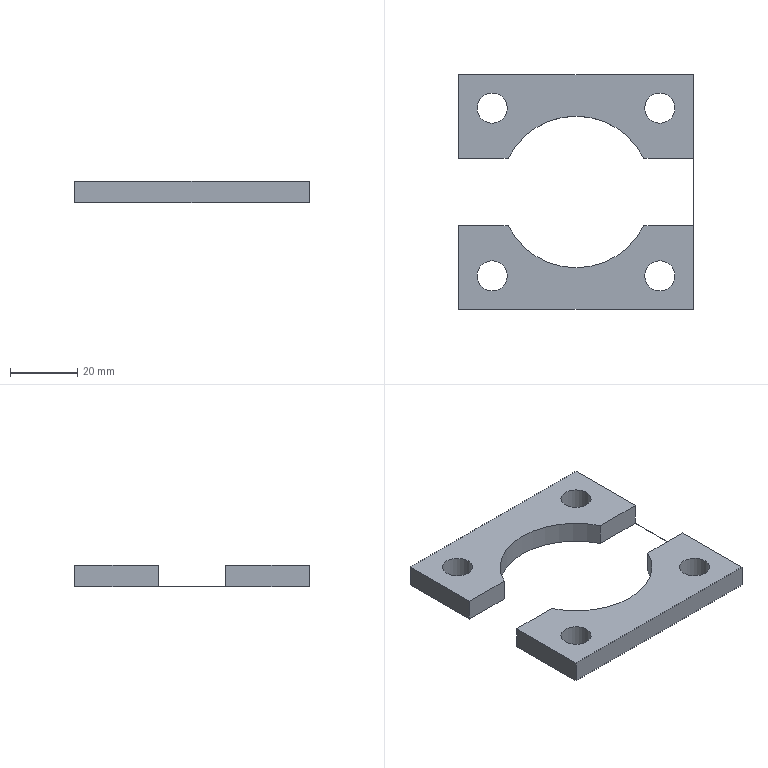Part | NX | features solid 2 | 1 solid | 20 faces | box 70 x 70 x 6.5 mm | volume 16344 mm3 | plane 14 | cylinder 6 | commonest cylinder face diameters 9 x4 45.2 x2
STEP:
#1=CARTESIAN_POINT('',(-460.,-390.,-210.));
#2=VERTEX_POINT('',#1);
#3=CARTESIAN_POINT('',(-390.,-390.,-210.));
#4=VERTEX_POINT('',#3);
#5=CARTESIAN_POINT('',(-460.,-390.,-210.));
#6=DIRECTION('',(1.,0.,0.));
#7=VECTOR('',#6,1000.);
#8=LINE('',#5,#7);
#9=EDGE_CURVE('',#2,#4,#8,.T.);
#10=ORIENTED_EDGE('',*,*,#9,.T.);
#11=CARTESIAN_POINT('',(-390.,-390.,-203.5));
#12=VERTEX_POINT('',#11);
#13=CARTESIAN_POINT('',(-390.,-390.,-203.5));
#14=DIRECTION('',(0.,0.,-1.));
#15=VECTOR('',#14,1000.);
#16=LINE('',#13,#15);
#17=EDGE_CURVE('',#12,#4,#16,.T.);
#18=ORIENTED_EDGE('',*,*,#17,.F.);
#19=CARTESIAN_POINT('',(-460.,-390.,-203.5));
#20=VERTEX_POINT('',#19);
#21=CARTESIAN_POINT('',(-460.,-390.,-203.5));
#22=DIRECTION('',(1.,0.,0.));
#23=VECTOR('',#22,1000.);
#24=LINE('',#21,#23);
#25=EDGE_CURVE('',#20,#12,#24,.T.);
#26=ORIENTED_EDGE('',*,*,#25,.F.);
#27=CARTESIAN_POINT('',(-460.,-390.,-203.5));
#28=DIRECTION('',(0.,0.,-1.));
#29=VECTOR('',#28,1000.);
#30=LINE('',#27,#29);
#31=EDGE_CURVE('',#20,#2,#30,.T.);
#32=ORIENTED_EDGE('',*,*,#31,.T.);
#33=EDGE_LOOP('',(#10,#18,#26,#32));
#34=FACE_BOUND('',#33,.T.);
#35=CARTESIAN_POINT('',(-460.,-390.,-203.5));
#36=DIRECTION('',(0.,1.,0.));
#37=DIRECTION('',(0.,0.,1.));
#38=AXIS2_PLACEMENT_3D('',#35,#36,#37);
#39=PLANE('',#38);
#40=ADVANCED_FACE('',(#34),#39,.F.);
#41=CARTESIAN_POINT('',(-390.,-320.,-210.));
#42=VERTEX_POINT('',#41);
#43=CARTESIAN_POINT('',(-390.,-390.,-210.));
#44=DIRECTION('',(0.,1.,0.));
#45=VECTOR('',#44,1000.);
#46=LINE('',#43,#45);
#47=EDGE_CURVE('',#4,#42,#46,.T.);
#48=ORIENTED_EDGE('',*,*,#47,.T.);
#49=CARTESIAN_POINT('',(-390.,-320.,-203.5));
#50=VERTEX_POINT('',#49);
#51=CARTESIAN_POINT('',(-390.,-320.,-210.));
#52=DIRECTION('',(0.,0.,-1.));
#53=VECTOR('',#52,1000.);
#54=LINE('',#51,#53);
#55=EDGE_CURVE('',#50,#42,#54,.T.);
#56=ORIENTED_EDGE('',*,*,#55,.F.);
#57=CARTESIAN_POINT('',(-390.,-345.,-203.5));
#58=VERTEX_POINT('',#57);
#59=CARTESIAN_POINT('',(-390.,-345.,-203.5));
#60=DIRECTION('',(0.,1.,0.));
#61=VECTOR('',#60,1000.);
#62=LINE('',#59,#61);
#63=EDGE_CURVE('',#58,#50,#62,.T.);
#64=ORIENTED_EDGE('',*,*,#63,.F.);
#65=CARTESIAN_POINT('',(-390.,-345.,-209.99));
#66=VERTEX_POINT('',#65);
#67=CARTESIAN_POINT('',(-390.,-345.,-203.5));
#68=DIRECTION('',(0.,0.,-1.));
#69=VECTOR('',#68,1000.);
#70=LINE('',#67,#69);
#71=EDGE_CURVE('',#58,#66,#70,.T.);
#72=ORIENTED_EDGE('',*,*,#71,.T.);
#73=CARTESIAN_POINT('',(-390.,-365.,-209.99));
#74=VERTEX_POINT('',#73);
#75=CARTESIAN_POINT('',(-390.,-390.,-209.99));
#76=DIRECTION('',(0.,-1.,0.));
#77=VECTOR('',#76,1000.);
#78=LINE('',#75,#77);
#79=EDGE_CURVE('',#74,#66,#78,.F.);
#80=ORIENTED_EDGE('',*,*,#79,.F.);
#81=CARTESIAN_POINT('',(-390.,-365.,-203.5));
#82=VERTEX_POINT('',#81);
#83=CARTESIAN_POINT('',(-390.,-365.,-203.5));
#84=DIRECTION('',(0.,0.,-1.));
#85=VECTOR('',#84,1000.);
#86=LINE('',#83,#85);
#87=EDGE_CURVE('',#82,#74,#86,.T.);
#88=ORIENTED_EDGE('',*,*,#87,.F.);
#89=CARTESIAN_POINT('',(-390.,-390.,-203.5));
#90=DIRECTION('',(0.,1.,0.));
#91=VECTOR('',#90,1000.);
#92=LINE('',#89,#91);
#93=EDGE_CURVE('',#12,#82,#92,.T.);
#94=ORIENTED_EDGE('',*,*,#93,.F.);
#95=ORIENTED_EDGE('',*,*,#17,.T.);
#96=EDGE_LOOP('',(#48,#56,#64,#72,#80,#88,#94,#95));
#97=FACE_BOUND('',#96,.T.);
#98=CARTESIAN_POINT('',(-390.,-390.,-203.5));
#99=DIRECTION('',(-1.,0.,0.));
#100=DIRECTION('',(0.,0.,-1.));
#101=AXIS2_PLACEMENT_3D('',#98,#99,#100);
#102=PLANE('',#101);
#103=ADVANCED_FACE('',(#97),#102,.F.);
#104=CARTESIAN_POINT('',(-390.01,-365.,-209.99));
#105=VERTEX_POINT('',#104);
#106=CARTESIAN_POINT('',(-390.,-365.,-209.99));
#107=DIRECTION('',(-1.,0.,0.));
#108=VECTOR('',#107,1000.);
#109=LINE('',#106,#108);
#110=EDGE_CURVE('',#74,#105,#109,.T.);
#111=ORIENTED_EDGE('',*,*,#110,.T.);
#112=CARTESIAN_POINT('',(-390.01,-365.,-210.));
#113=VERTEX_POINT('',#112);
#114=CARTESIAN_POINT('',(-390.01,-365.,-203.5));
#115=DIRECTION('',(0.,0.,1.));
#116=VECTOR('',#115,1000.);
#117=LINE('',#114,#116);
#118=EDGE_CURVE('',#105,#113,#117,.F.);
#119=ORIENTED_EDGE('',*,*,#118,.T.);
#120=CARTESIAN_POINT('',(-404.733,-365.,-210.));
#121=VERTEX_POINT('',#120);
#122=CARTESIAN_POINT('',(-390.,-365.,-210.));
#123=DIRECTION('',(-1.,0.,0.));
#124=VECTOR('',#123,1000.);
#125=LINE('',#122,#124);
#126=EDGE_CURVE('',#113,#121,#125,.T.);
#127=ORIENTED_EDGE('',*,*,#126,.T.);
#128=CARTESIAN_POINT('',(-404.733,-365.,-203.5));
#129=VERTEX_POINT('',#128);
#130=CARTESIAN_POINT('',(-404.733,-365.,-203.5));
#131=DIRECTION('',(0.,0.,-1.));
#132=VECTOR('',#131,1000.);
#133=LINE('',#130,#132);
#134=EDGE_CURVE('',#129,#121,#133,.T.);
#135=ORIENTED_EDGE('',*,*,#134,.F.);
#136=CARTESIAN_POINT('',(-390.,-365.,-203.5));
#137=DIRECTION('',(-1.,0.,0.));
#138=VECTOR('',#137,1000.);
#139=LINE('',#136,#138);
#140=EDGE_CURVE('',#82,#129,#139,.T.);
#141=ORIENTED_EDGE('',*,*,#140,.F.);
#142=ORIENTED_EDGE('',*,*,#87,.T.);
#143=EDGE_LOOP('',(#111,#119,#127,#135,#141,#142));
#144=FACE_BOUND('',#143,.T.);
#145=CARTESIAN_POINT('',(-390.,-365.,-203.5));
#146=DIRECTION('',(0.,-1.,0.));
#147=DIRECTION('',(1.,0.,0.));
#148=AXIS2_PLACEMENT_3D('',#145,#146,#147);
#149=PLANE('',#148);
#150=ADVANCED_FACE('',(#144),#149,.F.);
#151=CARTESIAN_POINT('',(-445.267,-365.,-210.));
#152=VERTEX_POINT('',#151);
#153=CARTESIAN_POINT('',(-425.,-355.,-210.));
#154=DIRECTION('',(0.,0.,1.));
#155=DIRECTION('',(0.,-1.,0.));
#156=AXIS2_PLACEMENT_3D('',#153,#154,#155);
#157=CIRCLE('',#156,22.6);
#158=EDGE_CURVE('',#152,#121,#157,.T.);
#159=ORIENTED_EDGE('',*,*,#158,.F.);
#160=CARTESIAN_POINT('',(-445.267,-365.,-203.5));
#161=VERTEX_POINT('',#160);
#162=CARTESIAN_POINT('',(-445.267,-365.,-203.5));
#163=DIRECTION('',(0.,0.,-1.));
#164=VECTOR('',#163,1000.);
#165=LINE('',#162,#164);
#166=EDGE_CURVE('',#161,#152,#165,.T.);
#167=ORIENTED_EDGE('',*,*,#166,.F.);
#168=CARTESIAN_POINT('',(-425.,-355.,-203.5));
#169=DIRECTION('',(0.,0.,1.));
#170=DIRECTION('',(0.,-1.,0.));
#171=AXIS2_PLACEMENT_3D('',#168,#169,#170);
#172=CIRCLE('',#171,22.6);
#173=EDGE_CURVE('',#161,#129,#172,.T.);
#174=ORIENTED_EDGE('',*,*,#173,.T.);
#175=ORIENTED_EDGE('',*,*,#134,.T.);
#176=EDGE_LOOP('',(#159,#167,#174,#175));
#177=FACE_BOUND('',#176,.T.);
#178=CARTESIAN_POINT('',(-425.,-355.,-203.5));
#179=DIRECTION('',(0.,0.,-1.));
#180=DIRECTION('',(0.,1.,0.));
#181=AXIS2_PLACEMENT_3D('',#178,#179,#180);
#182=CYLINDRICAL_SURFACE('',#181,22.6);
#183=ADVANCED_FACE('',(#177),#182,.F.);
#184=CARTESIAN_POINT('',(-460.,-365.,-210.));
#185=VERTEX_POINT('',#184);
#186=CARTESIAN_POINT('',(-445.267,-365.,-210.));
#187=DIRECTION('',(-1.,0.,0.));
#188=VECTOR('',#187,1000.);
#189=LINE('',#186,#188);
#190=EDGE_CURVE('',#152,#185,#189,.T.);
#191=ORIENTED_EDGE('',*,*,#190,.T.);
#192=CARTESIAN_POINT('',(-460.,-365.,-203.5));
#193=VERTEX_POINT('',#192);
#194=CARTESIAN_POINT('',(-460.,-365.,-203.5));
#195=DIRECTION('',(0.,0.,-1.));
#196=VECTOR('',#195,1000.);
#197=LINE('',#194,#196);
#198=EDGE_CURVE('',#193,#185,#197,.T.);
#199=ORIENTED_EDGE('',*,*,#198,.F.);
#200=CARTESIAN_POINT('',(-445.267,-365.,-203.5));
#201=DIRECTION('',(-1.,0.,0.));
#202=VECTOR('',#201,1000.);
#203=LINE('',#200,#202);
#204=EDGE_CURVE('',#161,#193,#203,.T.);
#205=ORIENTED_EDGE('',*,*,#204,.F.);
#206=ORIENTED_EDGE('',*,*,#166,.T.);
#207=EDGE_LOOP('',(#191,#199,#205,#206));
#208=FACE_BOUND('',#207,.T.);
#209=CARTESIAN_POINT('',(-445.267,-365.,-203.5));
#210=DIRECTION('',(0.,-1.,0.));
#211=DIRECTION('',(1.,0.,0.));
#212=AXIS2_PLACEMENT_3D('',#209,#210,#211);
#213=PLANE('',#212);
#214=ADVANCED_FACE('',(#208),#213,.F.);
#215=CARTESIAN_POINT('',(-450.,-384.5,-203.5));
#216=VERTEX_POINT('',#215);
#217=CARTESIAN_POINT('',(-450.,-380.,-203.5));
#218=DIRECTION('',(0.,0.,1.));
#219=DIRECTION('',(0.,-1.,0.));
#220=AXIS2_PLACEMENT_3D('',#217,#218,#219);
#221=CIRCLE('',#220,4.5);
#222=EDGE_CURVE('',#216,#216,#221,.T.);
#223=ORIENTED_EDGE('',*,*,#222,.T.);
#224=EDGE_LOOP('',(#223));
#225=FACE_BOUND('',#224,.T.);
#226=CARTESIAN_POINT('',(-450.,-384.5,-210.));
#227=VERTEX_POINT('',#226);
#228=CARTESIAN_POINT('',(-450.,-380.,-210.));
#229=DIRECTION('',(0.,0.,1.));
#230=DIRECTION('',(0.,-1.,0.));
#231=AXIS2_PLACEMENT_3D('',#228,#229,#230);
#232=CIRCLE('',#231,4.5);
#233=EDGE_CURVE('',#227,#227,#232,.T.);
#234=ORIENTED_EDGE('',*,*,#233,.F.);
#235=EDGE_LOOP('',(#234));
#236=FACE_BOUND('',#235,.T.);
#237=CARTESIAN_POINT('',(-450.,-380.,-203.5));
#238=DIRECTION('',(0.,0.,-1.));
#239=DIRECTION('',(0.,1.,0.));
#240=AXIS2_PLACEMENT_3D('',#237,#238,#239);
#241=CYLINDRICAL_SURFACE('',#240,4.5);
#242=ADVANCED_FACE('',(#225,#236),#241,.F.);
#243=CARTESIAN_POINT('',(-400.,-384.5,-203.5));
#244=VERTEX_POINT('',#243);
#245=CARTESIAN_POINT('',(-400.,-380.,-203.5));
#246=DIRECTION('',(0.,0.,1.));
#247=DIRECTION('',(0.,-1.,0.));
#248=AXIS2_PLACEMENT_3D('',#245,#246,#247);
#249=CIRCLE('',#248,4.5);
#250=EDGE_CURVE('',#244,#244,#249,.T.);
#251=ORIENTED_EDGE('',*,*,#250,.T.);
#252=EDGE_LOOP('',(#251));
#253=FACE_BOUND('',#252,.T.);
#254=CARTESIAN_POINT('',(-400.,-384.5,-210.));
#255=VERTEX_POINT('',#254);
#256=CARTESIAN_POINT('',(-400.,-380.,-210.));
#257=DIRECTION('',(0.,0.,1.));
#258=DIRECTION('',(0.,-1.,0.));
#259=AXIS2_PLACEMENT_3D('',#256,#257,#258);
#260=CIRCLE('',#259,4.5);
#261=EDGE_CURVE('',#255,#255,#260,.T.);
#262=ORIENTED_EDGE('',*,*,#261,.F.);
#263=EDGE_LOOP('',(#262));
#264=FACE_BOUND('',#263,.T.);
#265=CARTESIAN_POINT('',(-400.,-380.,-203.5));
#266=DIRECTION('',(0.,0.,-1.));
#267=DIRECTION('',(0.,1.,0.));
#268=AXIS2_PLACEMENT_3D('',#265,#266,#267);
#269=CYLINDRICAL_SURFACE('',#268,4.5);
#270=ADVANCED_FACE('',(#253,#264),#269,.F.);
#271=CARTESIAN_POINT('',(-460.,-365.,-210.));
#272=DIRECTION('',(0.,-1.,0.));
#273=VECTOR('',#272,1000.);
#274=LINE('',#271,#273);
#275=EDGE_CURVE('',#185,#2,#274,.T.);
#276=ORIENTED_EDGE('',*,*,#275,.T.);
#277=ORIENTED_EDGE('',*,*,#31,.F.);
#278=CARTESIAN_POINT('',(-460.,-365.,-203.5));
#279=DIRECTION('',(0.,-1.,0.));
#280=VECTOR('',#279,1000.);
#281=LINE('',#278,#280);
#282=EDGE_CURVE('',#193,#20,#281,.T.);
#283=ORIENTED_EDGE('',*,*,#282,.F.);
#284=ORIENTED_EDGE('',*,*,#198,.T.);
#285=EDGE_LOOP('',(#276,#277,#283,#284));
#286=FACE_BOUND('',#285,.T.);
#287=CARTESIAN_POINT('',(-460.,-365.,-203.5));
#288=DIRECTION('',(1.,0.,0.));
#289=DIRECTION('',(0.,0.,1.));
#290=AXIS2_PLACEMENT_3D('',#287,#288,#289);
#291=PLANE('',#290);
#292=ADVANCED_FACE('',(#286),#291,.F.);
#293=ORIENTED_EDGE('',*,*,#250,.F.);
#294=EDGE_LOOP('',(#293));
#295=FACE_BOUND('',#294,.T.);
#296=ORIENTED_EDGE('',*,*,#222,.F.);
#297=EDGE_LOOP('',(#296));
#298=FACE_BOUND('',#297,.T.);
#299=ORIENTED_EDGE('',*,*,#25,.T.);
#300=ORIENTED_EDGE('',*,*,#93,.T.);
#301=ORIENTED_EDGE('',*,*,#140,.T.);
#302=ORIENTED_EDGE('',*,*,#173,.F.);
#303=ORIENTED_EDGE('',*,*,#204,.T.);
#304=ORIENTED_EDGE('',*,*,#282,.T.);
#305=EDGE_LOOP('',(#299,#300,#301,#302,#303,#304));
#306=FACE_BOUND('',#305,.T.);
#307=CARTESIAN_POINT('',(-425.,-355.,-203.5));
#308=DIRECTION('',(0.,0.,1.));
#309=DIRECTION('',(0.,-1.,0.));
#310=AXIS2_PLACEMENT_3D('',#307,#308,#309);
#311=PLANE('',#310);
#312=ADVANCED_FACE('',(#295,#298,#306),#311,.T.);
#313=ORIENTED_EDGE('',*,*,#261,.T.);
#314=EDGE_LOOP('',(#313));
#315=FACE_BOUND('',#314,.T.);
#316=ORIENTED_EDGE('',*,*,#233,.T.);
#317=EDGE_LOOP('',(#316));
#318=FACE_BOUND('',#317,.T.);
#319=CARTESIAN_POINT('',(-390.01,-345.,-210.));
#320=VERTEX_POINT('',#319);
#321=CARTESIAN_POINT('',(-390.01,-390.,-210.));
#322=DIRECTION('',(0.,1.,0.));
#323=VECTOR('',#322,1000.);
#324=LINE('',#321,#323);
#325=EDGE_CURVE('',#113,#320,#324,.T.);
#326=ORIENTED_EDGE('',*,*,#325,.T.);
#327=CARTESIAN_POINT('',(-404.733,-345.,-210.));
#328=VERTEX_POINT('',#327);
#329=CARTESIAN_POINT('',(-390.,-345.,-210.));
#330=DIRECTION('',(-1.,0.,0.));
#331=VECTOR('',#330,1000.);
#332=LINE('',#329,#331);
#333=EDGE_CURVE('',#320,#328,#332,.T.);
#334=ORIENTED_EDGE('',*,*,#333,.T.);
#335=CARTESIAN_POINT('',(-445.267,-345.,-210.));
#336=VERTEX_POINT('',#335);
#337=CARTESIAN_POINT('',(-425.,-355.,-210.));
#338=DIRECTION('',(0.,0.,1.));
#339=DIRECTION('',(0.,-1.,0.));
#340=AXIS2_PLACEMENT_3D('',#337,#338,#339);
#341=CIRCLE('',#340,22.6);
#342=EDGE_CURVE('',#328,#336,#341,.T.);
#343=ORIENTED_EDGE('',*,*,#342,.T.);
#344=CARTESIAN_POINT('',(-460.,-345.,-210.));
#345=VERTEX_POINT('',#344);
#346=CARTESIAN_POINT('',(-445.267,-345.,-210.));
#347=DIRECTION('',(-1.,0.,0.));
#348=VECTOR('',#347,1000.);
#349=LINE('',#346,#348);
#350=EDGE_CURVE('',#336,#345,#349,.T.);
#351=ORIENTED_EDGE('',*,*,#350,.T.);
#352=CARTESIAN_POINT('',(-460.,-320.,-210.));
#353=VERTEX_POINT('',#352);
#354=CARTESIAN_POINT('',(-460.,-320.,-210.));
#355=DIRECTION('',(0.,-1.,0.));
#356=VECTOR('',#355,1000.);
#357=LINE('',#354,#356);
#358=EDGE_CURVE('',#353,#345,#357,.T.);
#359=ORIENTED_EDGE('',*,*,#358,.F.);
#360=CARTESIAN_POINT('',(-390.,-320.,-210.));
#361=DIRECTION('',(-1.,0.,0.));
#362=VECTOR('',#361,1000.);
#363=LINE('',#360,#362);
#364=EDGE_CURVE('',#42,#353,#363,.T.);
#365=ORIENTED_EDGE('',*,*,#364,.F.);
#366=ORIENTED_EDGE('',*,*,#47,.F.);
#367=ORIENTED_EDGE('',*,*,#9,.F.);
#368=ORIENTED_EDGE('',*,*,#275,.F.);
#369=ORIENTED_EDGE('',*,*,#190,.F.);
#370=ORIENTED_EDGE('',*,*,#158,.T.);
#371=ORIENTED_EDGE('',*,*,#126,.F.);
#372=EDGE_LOOP('',(#326,#334,#343,#351,#359,#365,#366,#367,#368,#369,#370,#371));
#373=FACE_BOUND('',#372,.T.);
#374=CARTESIAN_POINT('',(-400.,-334.5,-210.));
#375=VERTEX_POINT('',#374);
#376=CARTESIAN_POINT('',(-400.,-330.,-210.));
#377=DIRECTION('',(0.,0.,1.));
#378=DIRECTION('',(0.,-1.,0.));
#379=AXIS2_PLACEMENT_3D('',#376,#377,#378);
#380=CIRCLE('',#379,4.5);
#381=EDGE_CURVE('',#375,#375,#380,.T.);
#382=ORIENTED_EDGE('',*,*,#381,.T.);
#383=EDGE_LOOP('',(#382));
#384=FACE_BOUND('',#383,.T.);
#385=CARTESIAN_POINT('',(-450.,-334.5,-210.));
#386=VERTEX_POINT('',#385);
#387=CARTESIAN_POINT('',(-450.,-330.,-210.));
#388=DIRECTION('',(0.,0.,1.));
#389=DIRECTION('',(0.,-1.,0.));
#390=AXIS2_PLACEMENT_3D('',#387,#388,#389);
#391=CIRCLE('',#390,4.5);
#392=EDGE_CURVE('',#386,#386,#391,.T.);
#393=ORIENTED_EDGE('',*,*,#392,.T.);
#394=EDGE_LOOP('',(#393));
#395=FACE_BOUND('',#394,.T.);
#396=CARTESIAN_POINT('',(-425.,-355.,-210.));
#397=DIRECTION('',(0.,0.,1.));
#398=DIRECTION('',(0.,-1.,0.));
#399=AXIS2_PLACEMENT_3D('',#396,#397,#398);
#400=PLANE('',#399);
#401=ADVANCED_FACE('',(#315,#318,#373,#384,#395),#400,.F.);
#402=CARTESIAN_POINT('',(-390.01,-345.,-209.99));
#403=VERTEX_POINT('',#402);
#404=CARTESIAN_POINT('',(-390.,-345.,-209.99));
#405=DIRECTION('',(1.,0.,0.));
#406=VECTOR('',#405,1000.);
#407=LINE('',#404,#406);
#408=EDGE_CURVE('',#403,#66,#407,.T.);
#409=ORIENTED_EDGE('',*,*,#408,.F.);
#410=CARTESIAN_POINT('',(-390.01,-390.,-209.99));
#411=DIRECTION('',(0.,-1.,0.));
#412=VECTOR('',#411,1000.);
#413=LINE('',#410,#412);
#414=EDGE_CURVE('',#105,#403,#413,.F.);
#415=ORIENTED_EDGE('',*,*,#414,.F.);
#416=ORIENTED_EDGE('',*,*,#110,.F.);
#417=ORIENTED_EDGE('',*,*,#79,.T.);
#418=EDGE_LOOP('',(#409,#415,#416,#417));
#419=FACE_BOUND('',#418,.T.);
#420=CARTESIAN_POINT('',(-390.,-390.,-209.99));
#421=DIRECTION('',(0.,0.,1.));
#422=DIRECTION('',(0.,-1.,0.));
#423=AXIS2_PLACEMENT_3D('',#420,#421,#422);
#424=PLANE('',#423);
#425=ADVANCED_FACE('',(#419),#424,.T.);
#426=CARTESIAN_POINT('',(-390.01,-345.,-210.));
#427=DIRECTION('',(0.,0.,-1.));
#428=VECTOR('',#427,1000.);
#429=LINE('',#426,#428);
#430=EDGE_CURVE('',#320,#403,#429,.F.);
#431=ORIENTED_EDGE('',*,*,#430,.F.);
#432=ORIENTED_EDGE('',*,*,#325,.F.);
#433=ORIENTED_EDGE('',*,*,#118,.F.);
#434=ORIENTED_EDGE('',*,*,#414,.T.);
#435=EDGE_LOOP('',(#431,#432,#433,#434));
#436=FACE_BOUND('',#435,.T.);
#437=CARTESIAN_POINT('',(-390.01,-390.,-210.));
#438=DIRECTION('',(1.,0.,0.));
#439=DIRECTION('',(0.,1.,0.));
#440=AXIS2_PLACEMENT_3D('',#437,#438,#439);
#441=PLANE('',#440);
#442=ADVANCED_FACE('',(#436),#441,.F.);
#443=CARTESIAN_POINT('',(-460.,-320.,-203.5));
#444=VERTEX_POINT('',#443);
#445=CARTESIAN_POINT('',(-390.,-320.,-203.5));
#446=DIRECTION('',(-1.,0.,0.));
#447=VECTOR('',#446,1000.);
#448=LINE('',#445,#447);
#449=EDGE_CURVE('',#50,#444,#448,.T.);
#450=ORIENTED_EDGE('',*,*,#449,.F.);
#451=ORIENTED_EDGE('',*,*,#55,.T.);
#452=ORIENTED_EDGE('',*,*,#364,.T.);
#453=CARTESIAN_POINT('',(-460.,-320.,-203.5));
#454=DIRECTION('',(0.,0.,-1.));
#455=VECTOR('',#454,1000.);
#456=LINE('',#453,#455);
#457=EDGE_CURVE('',#444,#353,#456,.T.);
#458=ORIENTED_EDGE('',*,*,#457,.F.);
#459=EDGE_LOOP('',(#450,#451,#452,#458));
#460=FACE_BOUND('',#459,.T.);
#461=CARTESIAN_POINT('',(-390.,-320.,-210.));
#462=DIRECTION('',(0.,1.,0.));
#463=DIRECTION('',(-1.,0.,0.));
#464=AXIS2_PLACEMENT_3D('',#461,#462,#463);
#465=PLANE('',#464);
#466=ADVANCED_FACE('',(#460),#465,.T.);
#467=ORIENTED_EDGE('',*,*,#350,.F.);
#468=CARTESIAN_POINT('',(-445.267,-345.,-203.5));
#469=VERTEX_POINT('',#468);
#470=CARTESIAN_POINT('',(-445.267,-345.,-203.5));
#471=DIRECTION('',(0.,0.,-1.));
#472=VECTOR('',#471,1000.);
#473=LINE('',#470,#472);
#474=EDGE_CURVE('',#469,#336,#473,.T.);
#475=ORIENTED_EDGE('',*,*,#474,.F.);
#476=CARTESIAN_POINT('',(-460.,-345.,-203.5));
#477=VERTEX_POINT('',#476);
#478=CARTESIAN_POINT('',(-445.267,-345.,-203.5));
#479=DIRECTION('',(-1.,0.,0.));
#480=VECTOR('',#479,1000.);
#481=LINE('',#478,#480);
#482=EDGE_CURVE('',#469,#477,#481,.T.);
#483=ORIENTED_EDGE('',*,*,#482,.T.);
#484=CARTESIAN_POINT('',(-460.,-345.,-203.5));
#485=DIRECTION('',(0.,0.,-1.));
#486=VECTOR('',#485,1000.);
#487=LINE('',#484,#486);
#488=EDGE_CURVE('',#477,#345,#487,.T.);
#489=ORIENTED_EDGE('',*,*,#488,.T.);
#490=EDGE_LOOP('',(#467,#475,#483,#489));
#491=FACE_BOUND('',#490,.T.);
#492=CARTESIAN_POINT('',(-445.267,-345.,-203.5));
#493=DIRECTION('',(0.,-1.,0.));
#494=DIRECTION('',(1.,0.,0.));
#495=AXIS2_PLACEMENT_3D('',#492,#493,#494);
#496=PLANE('',#495);
#497=ADVANCED_FACE('',(#491),#496,.T.);
#498=ORIENTED_EDGE('',*,*,#358,.T.);
#499=ORIENTED_EDGE('',*,*,#488,.F.);
#500=CARTESIAN_POINT('',(-460.,-320.,-203.5));
#501=DIRECTION('',(0.,-1.,0.));
#502=VECTOR('',#501,1000.);
#503=LINE('',#500,#502);
#504=EDGE_CURVE('',#444,#477,#503,.T.);
#505=ORIENTED_EDGE('',*,*,#504,.F.);
#506=ORIENTED_EDGE('',*,*,#457,.T.);
#507=EDGE_LOOP('',(#498,#499,#505,#506));
#508=FACE_BOUND('',#507,.T.);
#509=CARTESIAN_POINT('',(-460.,-320.,-203.5));
#510=DIRECTION('',(1.,0.,0.));
#511=DIRECTION('',(0.,0.,1.));
#512=AXIS2_PLACEMENT_3D('',#509,#510,#511);
#513=PLANE('',#512);
#514=ADVANCED_FACE('',(#508),#513,.F.);
#515=ORIENTED_EDGE('',*,*,#430,.T.);
#516=ORIENTED_EDGE('',*,*,#408,.T.);
#517=ORIENTED_EDGE('',*,*,#71,.F.);
#518=CARTESIAN_POINT('',(-404.733,-345.,-203.5));
#519=VERTEX_POINT('',#518);
#520=CARTESIAN_POINT('',(-390.,-345.,-203.5));
#521=DIRECTION('',(-1.,0.,0.));
#522=VECTOR('',#521,1000.);
#523=LINE('',#520,#522);
#524=EDGE_CURVE('',#58,#519,#523,.T.);
#525=ORIENTED_EDGE('',*,*,#524,.T.);
#526=CARTESIAN_POINT('',(-404.733,-345.,-203.5));
#527=DIRECTION('',(0.,0.,-1.));
#528=VECTOR('',#527,1000.);
#529=LINE('',#526,#528);
#530=EDGE_CURVE('',#519,#328,#529,.T.);
#531=ORIENTED_EDGE('',*,*,#530,.T.);
#532=ORIENTED_EDGE('',*,*,#333,.F.);
#533=EDGE_LOOP('',(#515,#516,#517,#525,#531,#532));
#534=FACE_BOUND('',#533,.T.);
#535=CARTESIAN_POINT('',(-390.,-345.,-203.5));
#536=DIRECTION('',(0.,-1.,0.));
#537=DIRECTION('',(1.,0.,0.));
#538=AXIS2_PLACEMENT_3D('',#535,#536,#537);
#539=PLANE('',#538);
#540=ADVANCED_FACE('',(#534),#539,.T.);
#541=ORIENTED_EDGE('',*,*,#342,.F.);
#542=ORIENTED_EDGE('',*,*,#530,.F.);
#543=CARTESIAN_POINT('',(-425.,-355.,-203.5));
#544=DIRECTION('',(0.,0.,1.));
#545=DIRECTION('',(0.,-1.,0.));
#546=AXIS2_PLACEMENT_3D('',#543,#544,#545);
#547=CIRCLE('',#546,22.6);
#548=EDGE_CURVE('',#519,#469,#547,.T.);
#549=ORIENTED_EDGE('',*,*,#548,.T.);
#550=ORIENTED_EDGE('',*,*,#474,.T.);
#551=EDGE_LOOP('',(#541,#542,#549,#550));
#552=FACE_BOUND('',#551,.T.);
#553=CARTESIAN_POINT('',(-425.,-355.,-203.5));
#554=DIRECTION('',(0.,0.,-1.));
#555=DIRECTION('',(0.,1.,0.));
#556=AXIS2_PLACEMENT_3D('',#553,#554,#555);
#557=CYLINDRICAL_SURFACE('',#556,22.6);
#558=ADVANCED_FACE('',(#552),#557,.F.);
#559=CARTESIAN_POINT('',(-400.,-334.5,-203.5));
#560=VERTEX_POINT('',#559);
#561=CARTESIAN_POINT('',(-400.,-330.,-203.5));
#562=DIRECTION('',(0.,0.,1.));
#563=DIRECTION('',(0.,-1.,0.));
#564=AXIS2_PLACEMENT_3D('',#561,#562,#563);
#565=CIRCLE('',#564,4.5);
#566=EDGE_CURVE('',#560,#560,#565,.T.);
#567=ORIENTED_EDGE('',*,*,#566,.T.);
#568=EDGE_LOOP('',(#567));
#569=FACE_BOUND('',#568,.T.);
#570=ORIENTED_EDGE('',*,*,#381,.F.);
#571=EDGE_LOOP('',(#570));
#572=FACE_BOUND('',#571,.T.);
#573=CARTESIAN_POINT('',(-400.,-330.,-203.5));
#574=DIRECTION('',(0.,0.,-1.));
#575=DIRECTION('',(0.,1.,0.));
#576=AXIS2_PLACEMENT_3D('',#573,#574,#575);
#577=CYLINDRICAL_SURFACE('',#576,4.5);
#578=ADVANCED_FACE('',(#569,#572),#577,.F.);
#579=CARTESIAN_POINT('',(-450.,-334.5,-203.5));
#580=VERTEX_POINT('',#579);
#581=CARTESIAN_POINT('',(-450.,-330.,-203.5));
#582=DIRECTION('',(0.,0.,1.));
#583=DIRECTION('',(0.,-1.,0.));
#584=AXIS2_PLACEMENT_3D('',#581,#582,#583);
#585=CIRCLE('',#584,4.5);
#586=EDGE_CURVE('',#580,#580,#585,.T.);
#587=ORIENTED_EDGE('',*,*,#586,.T.);
#588=EDGE_LOOP('',(#587));
#589=FACE_BOUND('',#588,.T.);
#590=ORIENTED_EDGE('',*,*,#392,.F.);
#591=EDGE_LOOP('',(#590));
#592=FACE_BOUND('',#591,.T.);
#593=CARTESIAN_POINT('',(-450.,-330.,-203.5));
#594=DIRECTION('',(0.,0.,-1.));
#595=DIRECTION('',(0.,1.,0.));
#596=AXIS2_PLACEMENT_3D('',#593,#594,#595);
#597=CYLINDRICAL_SURFACE('',#596,4.5);
#598=ADVANCED_FACE('',(#589,#592),#597,.F.);
#599=ORIENTED_EDGE('',*,*,#566,.F.);
#600=EDGE_LOOP('',(#599));
#601=FACE_BOUND('',#600,.T.);
#602=ORIENTED_EDGE('',*,*,#482,.F.);
#603=ORIENTED_EDGE('',*,*,#548,.F.);
#604=ORIENTED_EDGE('',*,*,#524,.F.);
#605=ORIENTED_EDGE('',*,*,#63,.T.);
#606=ORIENTED_EDGE('',*,*,#449,.T.);
#607=ORIENTED_EDGE('',*,*,#504,.T.);
#608=EDGE_LOOP('',(#602,#603,#604,#605,#606,#607));
#609=FACE_BOUND('',#608,.T.);
#610=ORIENTED_EDGE('',*,*,#586,.F.);
#611=EDGE_LOOP('',(#610));
#612=FACE_BOUND('',#611,.T.);
#613=CARTESIAN_POINT('',(-425.,-355.,-203.5));
#614=DIRECTION('',(0.,0.,1.));
#615=DIRECTION('',(0.,-1.,0.));
#616=AXIS2_PLACEMENT_3D('',#613,#614,#615);
#617=PLANE('',#616);
#618=ADVANCED_FACE('',(#601,#609,#612),#617,.T.);
#619=CLOSED_SHELL('',(#40,#103,#150,#183,#214,#242,#270,#292,#312,#401,#425,#442,#466,#497,#514,#540,#558,#578,#598,#618));
#620=MANIFOLD_SOLID_BREP('',#619);
#621=(LENGTH_UNIT()NAMED_UNIT(*)SI_UNIT(.MILLI.,.METRE.));
#622=UNCERTAINTY_MEASURE_WITH_UNIT(LENGTH_MEASURE(0.00001),#621,'','');
#623=(NAMED_UNIT(*)PLANE_ANGLE_UNIT()SI_UNIT($,.RADIAN.));
#624=(NAMED_UNIT(*)SI_UNIT($,.STERADIAN.)SOLID_ANGLE_UNIT());
#625=(GEOMETRIC_REPRESENTATION_CONTEXT(3)GLOBAL_UNCERTAINTY_ASSIGNED_CONTEXT((#622))GLOBAL_UNIT_ASSIGNED_CONTEXT((#621,#623,#624))REPRESENTATION_CONTEXT('',''));
#626=ADVANCED_BREP_SHAPE_REPRESENTATION('',(#620),#625);